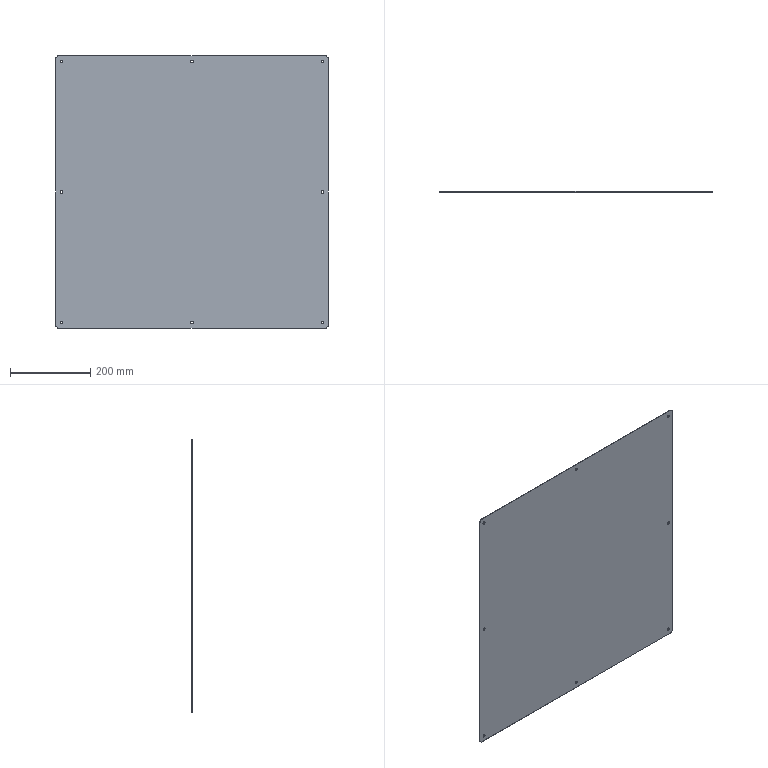Part | STEP file | 22-Cover plate | 1 solid | 26 faces | box 680 x 2 x 680 mm | volume 924081 mm3 | cylinder 20 | plane 6 | commonest cylinder face diameters 6.6 x16 20 x4